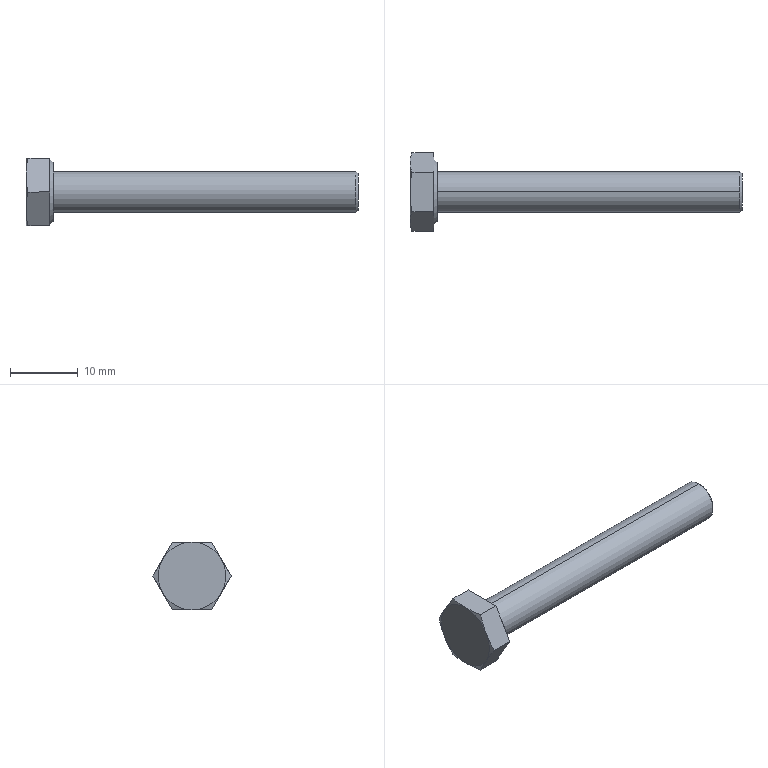Part | SolidWorks | features RevCut 3, Boss 1, Chamfer 1, Extrusion 1, Fillet 1, LPattern 1 | 1 solid | 22 faces | box 49 x 11.547 x 10 mm | volume 1608 mm3 | cone 10 | plane 10 | cylinder 2 | commonest cylinder face diameters 6 x2
STEP:
#1=CARTESIAN_POINT('',(49.,0.,-2.7));
#2=VERTEX_POINT('',#1);
#3=CARTESIAN_POINT('',(49.,0.,2.7));
#4=VERTEX_POINT('',#3);
#5=CARTESIAN_POINT('',(49.,0.,0.));
#6=DIRECTION('',(1.,0.,0.));
#7=DIRECTION('',(0.,0.,-1.));
#8=AXIS2_PLACEMENT_3D('',#5,#6,#7);
#9=CIRCLE('',#8,2.7);
#10=EDGE_CURVE('',#2,#4,#9,.T.);
#11=ORIENTED_EDGE('',*,*,#10,.F.);
#12=CARTESIAN_POINT('',(48.7,0.,-3.));
#13=VERTEX_POINT('',#12);
#14=CARTESIAN_POINT('',(49.,0.,-2.7));
#15=DIRECTION('',(-0.7071,0.,-0.7071));
#16=VECTOR('',#15,1000.);
#17=LINE('',#14,#16);
#18=EDGE_CURVE('',#2,#13,#17,.T.);
#19=ORIENTED_EDGE('',*,*,#18,.T.);
#20=CARTESIAN_POINT('',(48.7,0.,3.));
#21=VERTEX_POINT('',#20);
#22=CARTESIAN_POINT('',(48.7,0.,0.));
#23=DIRECTION('',(-1.,0.,0.));
#24=DIRECTION('',(0.,0.,-1.));
#25=AXIS2_PLACEMENT_3D('',#22,#23,#24);
#26=CIRCLE('',#25,3.);
#27=EDGE_CURVE('',#21,#13,#26,.T.);
#28=ORIENTED_EDGE('',*,*,#27,.F.);
#29=CARTESIAN_POINT('',(49.,0.,2.7));
#30=DIRECTION('',(-0.7071,0.,0.7071));
#31=VECTOR('',#30,1000.);
#32=LINE('',#29,#31);
#33=EDGE_CURVE('',#4,#21,#32,.T.);
#34=ORIENTED_EDGE('',*,*,#33,.F.);
#35=EDGE_LOOP('',(#11,#19,#28,#34));
#36=FACE_OUTER_BOUND('',#35,.T.);
#37=CARTESIAN_POINT('',(49.,0.,0.));
#38=DIRECTION('',(-1.,0.,0.));
#39=DIRECTION('',(0.,0.,1.));
#40=AXIS2_PLACEMENT_3D('',#37,#38,#39);
#41=CONICAL_SURFACE('',#40,2.7,0.7854);
#42=ADVANCED_FACE('',(#36),#41,.T.);
#43=ORIENTED_EDGE('',*,*,#27,.T.);
#44=CARTESIAN_POINT('',(4.,0.,-3.));
#45=VERTEX_POINT('',#44);
#46=CARTESIAN_POINT('',(49.,0.,-3.));
#47=DIRECTION('',(-1.,0.,0.));
#48=VECTOR('',#47,1000.);
#49=LINE('',#46,#48);
#50=EDGE_CURVE('',#13,#45,#49,.T.);
#51=ORIENTED_EDGE('',*,*,#50,.T.);
#52=CARTESIAN_POINT('',(4.,0.,3.));
#53=VERTEX_POINT('',#52);
#54=CARTESIAN_POINT('',(4.,0.,0.));
#55=DIRECTION('',(1.,0.,0.));
#56=DIRECTION('',(0.,0.,1.));
#57=AXIS2_PLACEMENT_3D('',#54,#55,#56);
#58=CIRCLE('',#57,3.);
#59=EDGE_CURVE('',#45,#53,#58,.T.);
#60=ORIENTED_EDGE('',*,*,#59,.T.);
#61=CARTESIAN_POINT('',(49.,0.,3.));
#62=DIRECTION('',(-1.,0.,0.));
#63=VECTOR('',#62,1000.);
#64=LINE('',#61,#63);
#65=EDGE_CURVE('',#21,#53,#64,.T.);
#66=ORIENTED_EDGE('',*,*,#65,.F.);
#67=EDGE_LOOP('',(#43,#51,#60,#66));
#68=FACE_OUTER_BOUND('',#67,.T.);
#69=CARTESIAN_POINT('',(49.,0.,0.));
#70=DIRECTION('',(-1.,0.,0.));
#71=DIRECTION('',(0.,0.,1.));
#72=AXIS2_PLACEMENT_3D('',#69,#70,#71);
#73=CYLINDRICAL_SURFACE('',#72,3.);
#74=ADVANCED_FACE('',(#68),#73,.T.);
#75=CARTESIAN_POINT('',(4.,0.,4.37));
#76=VERTEX_POINT('',#75);
#77=CARTESIAN_POINT('',(4.,0.,-4.37));
#78=VERTEX_POINT('',#77);
#79=CARTESIAN_POINT('',(4.,0.,0.));
#80=DIRECTION('',(-1.,0.,0.));
#81=DIRECTION('',(0.,0.,1.));
#82=AXIS2_PLACEMENT_3D('',#79,#80,#81);
#83=CIRCLE('',#82,4.37);
#84=EDGE_CURVE('',#76,#78,#83,.T.);
#85=ORIENTED_EDGE('',*,*,#84,.T.);
#86=CARTESIAN_POINT('',(3.5,0.,-4.87));
#87=VERTEX_POINT('',#86);
#88=CARTESIAN_POINT('',(3.5,0.,-4.87));
#89=DIRECTION('',(-0.7071,0.,-0.7071));
#90=VECTOR('',#89,1000.);
#91=LINE('',#88,#90);
#92=EDGE_CURVE('',#78,#87,#91,.T.);
#93=ORIENTED_EDGE('',*,*,#92,.T.);
#94=CARTESIAN_POINT('',(3.5,0.,4.87));
#95=VERTEX_POINT('',#94);
#96=CARTESIAN_POINT('',(3.5,0.,0.));
#97=DIRECTION('',(-1.,0.,0.));
#98=DIRECTION('',(0.,0.,1.));
#99=AXIS2_PLACEMENT_3D('',#96,#97,#98);
#100=CIRCLE('',#99,4.87);
#101=EDGE_CURVE('',#95,#87,#100,.T.);
#102=ORIENTED_EDGE('',*,*,#101,.F.);
#103=CARTESIAN_POINT('',(3.5,0.,4.87));
#104=DIRECTION('',(-0.7071,0.,0.7071));
#105=VECTOR('',#104,1000.);
#106=LINE('',#103,#105);
#107=EDGE_CURVE('',#76,#95,#106,.T.);
#108=ORIENTED_EDGE('',*,*,#107,.F.);
#109=EDGE_LOOP('',(#85,#93,#102,#108));
#110=FACE_OUTER_BOUND('',#109,.T.);
#111=CARTESIAN_POINT('',(3.5,0.,0.));
#112=DIRECTION('',(-1.,0.,0.));
#113=DIRECTION('',(0.,0.,1.));
#114=AXIS2_PLACEMENT_3D('',#111,#112,#113);
#115=CONICAL_SURFACE('',#114,4.87,0.7854);
#116=ADVANCED_FACE('',(#110),#115,.T.);
#117=ORIENTED_EDGE('',*,*,#84,.F.);
#118=CARTESIAN_POINT('',(4.,0.,0.));
#119=DIRECTION('',(-1.,0.,0.));
#120=DIRECTION('',(0.,0.,1.));
#121=AXIS2_PLACEMENT_3D('',#118,#119,#120);
#122=CIRCLE('',#121,4.37);
#123=EDGE_CURVE('',#78,#76,#122,.T.);
#124=ORIENTED_EDGE('',*,*,#123,.F.);
#125=EDGE_LOOP('',(#117,#124));
#126=FACE_OUTER_BOUND('',#125,.T.);
#127=CARTESIAN_POINT('',(4.,0.,0.));
#128=DIRECTION('',(1.,0.,0.));
#129=DIRECTION('',(0.,0.,1.));
#130=AXIS2_PLACEMENT_3D('',#127,#128,#129);
#131=CIRCLE('',#130,3.);
#132=EDGE_CURVE('',#53,#45,#131,.T.);
#133=ORIENTED_EDGE('',*,*,#132,.F.);
#134=ORIENTED_EDGE('',*,*,#59,.F.);
#135=EDGE_LOOP('',(#133,#134));
#136=FACE_BOUND('',#135,.T.);
#137=CARTESIAN_POINT('',(4.,-2.887,5.));
#138=DIRECTION('',(-1.,0.,0.));
#139=DIRECTION('',(0.,0.,1.));
#140=AXIS2_PLACEMENT_3D('',#137,#138,#139);
#141=PLANE('',#140);
#142=ADVANCED_FACE('',(#126,#136),#141,.F.);
#143=CARTESIAN_POINT('',(0.2815,-5.774,0.));
#144=VERTEX_POINT('',#143);
#145=CARTESIAN_POINT('',(0.,-4.33,2.5));
#146=VERTEX_POINT('',#145);
#147=CARTESIAN_POINT('',(0.2815,-5.774,0.));
#148=CARTESIAN_POINT('',(0.1064,-5.292,0.8333));
#149=CARTESIAN_POINT('',(0.,-4.811,1.667));
#150=CARTESIAN_POINT('',(0.,-4.33,2.5));
#151=B_SPLINE_CURVE_WITH_KNOTS('',3,(#147,#148,#149,#150),.UNSPECIFIED.,.F.,.F.,(4,4),(0.000000231,0.002887),.UNSPECIFIED.);
#152=EDGE_CURVE('',#144,#146,#151,.T.);
#153=ORIENTED_EDGE('',*,*,#152,.F.);
#154=CARTESIAN_POINT('',(3.5,-5.774,0.));
#155=VERTEX_POINT('',#154);
#156=CARTESIAN_POINT('',(4.,-5.774,0.));
#157=DIRECTION('',(-1.,0.,0.));
#158=VECTOR('',#157,1000.);
#159=LINE('',#156,#158);
#160=EDGE_CURVE('',#155,#144,#159,.T.);
#161=ORIENTED_EDGE('',*,*,#160,.F.);
#162=CARTESIAN_POINT('',(3.5,-2.887,5.));
#163=VERTEX_POINT('',#162);
#164=CARTESIAN_POINT('',(3.5,-2.887,5.));
#165=DIRECTION('',(0.,-0.5,-0.866));
#166=VECTOR('',#165,1000.);
#167=LINE('',#164,#166);
#168=EDGE_CURVE('',#163,#155,#167,.T.);
#169=ORIENTED_EDGE('',*,*,#168,.F.);
#170=CARTESIAN_POINT('',(0.2815,-2.887,5.));
#171=VERTEX_POINT('',#170);
#172=CARTESIAN_POINT('',(4.,-2.887,5.));
#173=DIRECTION('',(-1.,0.,0.));
#174=VECTOR('',#173,1000.);
#175=LINE('',#172,#174);
#176=EDGE_CURVE('',#163,#171,#175,.T.);
#177=ORIENTED_EDGE('',*,*,#176,.T.);
#178=CARTESIAN_POINT('',(0.,-4.33,2.5));
#179=CARTESIAN_POINT('',(0.,-3.849,3.333));
#180=CARTESIAN_POINT('',(0.1064,-3.368,4.167));
#181=CARTESIAN_POINT('',(0.2815,-2.887,5.));
#182=B_SPLINE_CURVE_WITH_KNOTS('',3,(#178,#179,#180,#181),.UNSPECIFIED.,.F.,.F.,(4,4),(0.002887,0.005774),.UNSPECIFIED.);
#183=EDGE_CURVE('',#146,#171,#182,.T.);
#184=ORIENTED_EDGE('',*,*,#183,.F.);
#185=EDGE_LOOP('',(#153,#161,#169,#177,#184));
#186=FACE_OUTER_BOUND('',#185,.T.);
#187=CARTESIAN_POINT('',(4.,-2.887,5.));
#188=DIRECTION('',(0.,0.866,-0.5));
#189=DIRECTION('',(0.,0.5,0.866));
#190=AXIS2_PLACEMENT_3D('',#187,#188,#189);
#191=PLANE('',#190);
#192=ADVANCED_FACE('',(#186),#191,.F.);
#193=CARTESIAN_POINT('',(0.2815,-2.887,-5.));
#194=VERTEX_POINT('',#193);
#195=CARTESIAN_POINT('',(0.,-4.33,-2.5));
#196=VERTEX_POINT('',#195);
#197=CARTESIAN_POINT('',(0.2815,-2.887,-5.));
#198=CARTESIAN_POINT('',(0.1064,-3.368,-4.167));
#199=CARTESIAN_POINT('',(0.,-3.849,-3.333));
#200=CARTESIAN_POINT('',(0.,-4.33,-2.5));
#201=B_SPLINE_CURVE_WITH_KNOTS('',3,(#197,#198,#199,#200),.UNSPECIFIED.,.F.,.F.,(4,4),(0.000000231,0.002887),.UNSPECIFIED.);
#202=EDGE_CURVE('',#194,#196,#201,.T.);
#203=ORIENTED_EDGE('',*,*,#202,.F.);
#204=CARTESIAN_POINT('',(3.5,-2.887,-5.));
#205=VERTEX_POINT('',#204);
#206=CARTESIAN_POINT('',(4.,-2.887,-5.));
#207=DIRECTION('',(-1.,0.,0.));
#208=VECTOR('',#207,1000.);
#209=LINE('',#206,#208);
#210=EDGE_CURVE('',#205,#194,#209,.T.);
#211=ORIENTED_EDGE('',*,*,#210,.F.);
#212=CARTESIAN_POINT('',(3.5,-5.774,0.));
#213=DIRECTION('',(0.,0.5,-0.866));
#214=VECTOR('',#213,1000.);
#215=LINE('',#212,#214);
#216=EDGE_CURVE('',#155,#205,#215,.T.);
#217=ORIENTED_EDGE('',*,*,#216,.F.);
#218=ORIENTED_EDGE('',*,*,#160,.T.);
#219=CARTESIAN_POINT('',(0.,-4.33,-2.5));
#220=CARTESIAN_POINT('',(0.,-4.811,-1.667));
#221=CARTESIAN_POINT('',(0.1064,-5.292,-0.8333));
#222=CARTESIAN_POINT('',(0.2815,-5.774,0.));
#223=B_SPLINE_CURVE_WITH_KNOTS('',3,(#219,#220,#221,#222),.UNSPECIFIED.,.F.,.F.,(4,4),(0.002887,0.005774),.UNSPECIFIED.);
#224=EDGE_CURVE('',#196,#144,#223,.T.);
#225=ORIENTED_EDGE('',*,*,#224,.F.);
#226=EDGE_LOOP('',(#203,#211,#217,#218,#225));
#227=FACE_OUTER_BOUND('',#226,.T.);
#228=CARTESIAN_POINT('',(4.,-5.774,0.));
#229=DIRECTION('',(0.,0.866,0.5));
#230=DIRECTION('',(0.,-0.5,0.866));
#231=AXIS2_PLACEMENT_3D('',#228,#229,#230);
#232=PLANE('',#231);
#233=ADVANCED_FACE('',(#227),#232,.F.);
#234=CARTESIAN_POINT('',(0.2815,2.887,-5.));
#235=VERTEX_POINT('',#234);
#236=CARTESIAN_POINT('',(0.,0.,-5.));
#237=VERTEX_POINT('',#236);
#238=CARTESIAN_POINT('',(0.2815,2.887,-5.));
#239=CARTESIAN_POINT('',(0.1069,1.927,-5.));
#240=CARTESIAN_POINT('',(0.,0.9642,-5.));
#241=CARTESIAN_POINT('',(0.,0.,-5.));
#242=B_SPLINE_CURVE_WITH_KNOTS('',3,(#238,#239,#240,#241),.UNSPECIFIED.,.F.,.F.,(4,4),(0.01041,0.01332),.UNSPECIFIED.);
#243=EDGE_CURVE('',#235,#237,#242,.T.);
#244=ORIENTED_EDGE('',*,*,#243,.F.);
#245=CARTESIAN_POINT('',(3.5,2.887,-5.));
#246=VERTEX_POINT('',#245);
#247=CARTESIAN_POINT('',(4.,2.887,-5.));
#248=DIRECTION('',(-1.,0.,0.));
#249=VECTOR('',#248,1000.);
#250=LINE('',#247,#249);
#251=EDGE_CURVE('',#246,#235,#250,.T.);
#252=ORIENTED_EDGE('',*,*,#251,.F.);
#253=CARTESIAN_POINT('',(3.5,-2.887,-5.));
#254=DIRECTION('',(0.,1.,0.));
#255=VECTOR('',#254,1000.);
#256=LINE('',#253,#255);
#257=EDGE_CURVE('',#205,#246,#256,.T.);
#258=ORIENTED_EDGE('',*,*,#257,.F.);
#259=ORIENTED_EDGE('',*,*,#210,.T.);
#260=CARTESIAN_POINT('',(0.,0.,-5.));
#261=CARTESIAN_POINT('',(0.,-0.4807,-5.));
#262=CARTESIAN_POINT('',(0.02571,-0.962,-5.));
#263=CARTESIAN_POINT('',(0.123,-1.926,-5.));
#264=CARTESIAN_POINT('',(0.1945,-2.409,-5.));
#265=CARTESIAN_POINT('',(0.2815,-2.887,-5.));
#266=B_SPLINE_CURVE_WITH_KNOTS('',3,(#260,#261,#262,#263,#264,#265),.UNSPECIFIED.,.F.,.F.,(4,2,4),(0.01332,0.01477,0.01622),.UNSPECIFIED.);
#267=EDGE_CURVE('',#237,#194,#266,.T.);
#268=ORIENTED_EDGE('',*,*,#267,.F.);
#269=EDGE_LOOP('',(#244,#252,#258,#259,#268));
#270=FACE_OUTER_BOUND('',#269,.T.);
#271=CARTESIAN_POINT('',(4.,-2.887,-5.));
#272=DIRECTION('',(0.,0.,1.));
#273=DIRECTION('',(0.,-1.,0.));
#274=AXIS2_PLACEMENT_3D('',#271,#272,#273);
#275=PLANE('',#274);
#276=ADVANCED_FACE('',(#270),#275,.F.);
#277=CARTESIAN_POINT('',(0.2815,5.774,0.));
#278=VERTEX_POINT('',#277);
#279=CARTESIAN_POINT('',(0.,4.33,-2.5));
#280=VERTEX_POINT('',#279);
#281=CARTESIAN_POINT('',(0.2815,5.774,0.));
#282=CARTESIAN_POINT('',(0.1064,5.292,-0.8333));
#283=CARTESIAN_POINT('',(0.,4.811,-1.667));
#284=CARTESIAN_POINT('',(0.,4.33,-2.5));
#285=B_SPLINE_CURVE_WITH_KNOTS('',3,(#281,#282,#283,#284),.UNSPECIFIED.,.F.,.F.,(4,4),(0.000000231,0.002887),.UNSPECIFIED.);
#286=EDGE_CURVE('',#278,#280,#285,.T.);
#287=ORIENTED_EDGE('',*,*,#286,.F.);
#288=CARTESIAN_POINT('',(3.5,5.774,0.));
#289=VERTEX_POINT('',#288);
#290=CARTESIAN_POINT('',(4.,5.774,0.));
#291=DIRECTION('',(-1.,0.,0.));
#292=VECTOR('',#291,1000.);
#293=LINE('',#290,#292);
#294=EDGE_CURVE('',#289,#278,#293,.T.);
#295=ORIENTED_EDGE('',*,*,#294,.F.);
#296=CARTESIAN_POINT('',(3.5,2.887,-5.));
#297=DIRECTION('',(0.,0.5,0.866));
#298=VECTOR('',#297,1000.);
#299=LINE('',#296,#298);
#300=EDGE_CURVE('',#246,#289,#299,.T.);
#301=ORIENTED_EDGE('',*,*,#300,.F.);
#302=ORIENTED_EDGE('',*,*,#251,.T.);
#303=CARTESIAN_POINT('',(0.,4.33,-2.5));
#304=CARTESIAN_POINT('',(0.,3.849,-3.333));
#305=CARTESIAN_POINT('',(0.1064,3.368,-4.167));
#306=CARTESIAN_POINT('',(0.2815,2.887,-5.));
#307=B_SPLINE_CURVE_WITH_KNOTS('',3,(#303,#304,#305,#306),.UNSPECIFIED.,.F.,.F.,(4,4),(0.002887,0.005774),.UNSPECIFIED.);
#308=EDGE_CURVE('',#280,#235,#307,.T.);
#309=ORIENTED_EDGE('',*,*,#308,.F.);
#310=EDGE_LOOP('',(#287,#295,#301,#302,#309));
#311=FACE_OUTER_BOUND('',#310,.T.);
#312=CARTESIAN_POINT('',(4.,2.887,-5.));
#313=DIRECTION('',(0.,-0.866,0.5));
#314=DIRECTION('',(0.,-0.5,-0.866));
#315=AXIS2_PLACEMENT_3D('',#312,#313,#314);
#316=PLANE('',#315);
#317=ADVANCED_FACE('',(#311),#316,.F.);
#318=CARTESIAN_POINT('',(0.2815,2.887,5.));
#319=VERTEX_POINT('',#318);
#320=CARTESIAN_POINT('',(0.,4.33,2.5));
#321=VERTEX_POINT('',#320);
#322=CARTESIAN_POINT('',(0.2815,2.887,5.));
#323=CARTESIAN_POINT('',(0.1064,3.368,4.167));
#324=CARTESIAN_POINT('',(0.,3.849,3.333));
#325=CARTESIAN_POINT('',(0.,4.33,2.5));
#326=B_SPLINE_CURVE_WITH_KNOTS('',3,(#322,#323,#324,#325),.UNSPECIFIED.,.F.,.F.,(4,4),(0.000000231,0.002887),.UNSPECIFIED.);
#327=EDGE_CURVE('',#319,#321,#326,.T.);
#328=ORIENTED_EDGE('',*,*,#327,.F.);
#329=CARTESIAN_POINT('',(3.5,2.887,5.));
#330=VERTEX_POINT('',#329);
#331=CARTESIAN_POINT('',(4.,2.887,5.));
#332=DIRECTION('',(-1.,0.,0.));
#333=VECTOR('',#332,1000.);
#334=LINE('',#331,#333);
#335=EDGE_CURVE('',#330,#319,#334,.T.);
#336=ORIENTED_EDGE('',*,*,#335,.F.);
#337=CARTESIAN_POINT('',(3.5,5.774,0.));
#338=DIRECTION('',(0.,-0.5,0.866));
#339=VECTOR('',#338,1000.);
#340=LINE('',#337,#339);
#341=EDGE_CURVE('',#289,#330,#340,.T.);
#342=ORIENTED_EDGE('',*,*,#341,.F.);
#343=ORIENTED_EDGE('',*,*,#294,.T.);
#344=CARTESIAN_POINT('',(0.,4.33,2.5));
#345=CARTESIAN_POINT('',(0.,4.811,1.667));
#346=CARTESIAN_POINT('',(0.1064,5.292,0.8333));
#347=CARTESIAN_POINT('',(0.2815,5.774,0.));
#348=B_SPLINE_CURVE_WITH_KNOTS('',3,(#344,#345,#346,#347),.UNSPECIFIED.,.F.,.F.,(4,4),(0.002887,0.005774),.UNSPECIFIED.);
#349=EDGE_CURVE('',#321,#278,#348,.T.);
#350=ORIENTED_EDGE('',*,*,#349,.F.);
#351=EDGE_LOOP('',(#328,#336,#342,#343,#350));
#352=FACE_OUTER_BOUND('',#351,.T.);
#353=CARTESIAN_POINT('',(4.,5.774,0.));
#354=DIRECTION('',(0.,-0.866,-0.5));
#355=DIRECTION('',(0.,0.5,-0.866));
#356=AXIS2_PLACEMENT_3D('',#353,#354,#355);
#357=PLANE('',#356);
#358=ADVANCED_FACE('',(#352),#357,.F.);
#359=CARTESIAN_POINT('',(0.,0.,5.));
#360=VERTEX_POINT('',#359);
#361=CARTESIAN_POINT('',(0.2815,-2.887,5.));
#362=CARTESIAN_POINT('',(0.1945,-2.409,5.));
#363=CARTESIAN_POINT('',(0.123,-1.926,5.));
#364=CARTESIAN_POINT('',(0.02571,-0.962,5.));
#365=CARTESIAN_POINT('',(0.,-0.4807,5.));
#366=CARTESIAN_POINT('',(0.,0.,5.));
#367=B_SPLINE_CURVE_WITH_KNOTS('',3,(#361,#362,#363,#364,#365,#366),.UNSPECIFIED.,.F.,.F.,(4,2,4),(0.004911,0.006366,0.00782),.UNSPECIFIED.);
#368=EDGE_CURVE('',#171,#360,#367,.T.);
#369=ORIENTED_EDGE('',*,*,#368,.F.);
#370=ORIENTED_EDGE('',*,*,#176,.F.);
#371=CARTESIAN_POINT('',(3.5,2.887,5.));
#372=DIRECTION('',(0.,-1.,0.));
#373=VECTOR('',#372,1000.);
#374=LINE('',#371,#373);
#375=EDGE_CURVE('',#330,#163,#374,.T.);
#376=ORIENTED_EDGE('',*,*,#375,.F.);
#377=ORIENTED_EDGE('',*,*,#335,.T.);
#378=CARTESIAN_POINT('',(0.,0.,5.));
#379=CARTESIAN_POINT('',(0.,0.9642,5.));
#380=CARTESIAN_POINT('',(0.1069,1.927,5.));
#381=CARTESIAN_POINT('',(0.2815,2.887,5.));
#382=B_SPLINE_CURVE_WITH_KNOTS('',3,(#378,#379,#380,#381),.UNSPECIFIED.,.F.,.F.,(4,4),(0.00782,0.01074),.UNSPECIFIED.);
#383=EDGE_CURVE('',#360,#319,#382,.T.);
#384=ORIENTED_EDGE('',*,*,#383,.F.);
#385=EDGE_LOOP('',(#369,#370,#376,#377,#384));
#386=FACE_OUTER_BOUND('',#385,.T.);
#387=CARTESIAN_POINT('',(4.,2.887,5.));
#388=DIRECTION('',(0.,0.,-1.));
#389=DIRECTION('',(0.,1.,0.));
#390=AXIS2_PLACEMENT_3D('',#387,#388,#389);
#391=PLANE('',#390);
#392=ADVANCED_FACE('',(#386),#391,.F.);
#393=ORIENTED_EDGE('',*,*,#101,.T.);
#394=CARTESIAN_POINT('',(3.5,0.,0.));
#395=DIRECTION('',(-1.,0.,0.));
#396=DIRECTION('',(0.,0.,1.));
#397=AXIS2_PLACEMENT_3D('',#394,#395,#396);
#398=CIRCLE('',#397,4.87);
#399=EDGE_CURVE('',#87,#95,#398,.T.);
#400=ORIENTED_EDGE('',*,*,#399,.T.);
#401=EDGE_LOOP('',(#393,#400));
#402=FACE_BOUND('',#401,.T.);
#403=ORIENTED_EDGE('',*,*,#168,.T.);
#404=ORIENTED_EDGE('',*,*,#216,.T.);
#405=ORIENTED_EDGE('',*,*,#257,.T.);
#406=ORIENTED_EDGE('',*,*,#300,.T.);
#407=ORIENTED_EDGE('',*,*,#341,.T.);
#408=ORIENTED_EDGE('',*,*,#375,.T.);
#409=EDGE_LOOP('',(#403,#404,#405,#406,#407,#408));
#410=FACE_OUTER_BOUND('',#409,.T.);
#411=CARTESIAN_POINT('',(3.5,4.87,0.));
#412=DIRECTION('',(1.,0.,0.));
#413=DIRECTION('',(0.,0.,-1.));
#414=AXIS2_PLACEMENT_3D('',#411,#412,#413);
#415=PLANE('',#414);
#416=ADVANCED_FACE('',(#402,#410),#415,.T.);
#417=ORIENTED_EDGE('',*,*,#92,.F.);
#418=ORIENTED_EDGE('',*,*,#123,.T.);
#419=ORIENTED_EDGE('',*,*,#107,.T.);
#420=ORIENTED_EDGE('',*,*,#399,.F.);
#421=EDGE_LOOP('',(#417,#418,#419,#420));
#422=FACE_OUTER_BOUND('',#421,.T.);
#423=CARTESIAN_POINT('',(3.5,0.,0.));
#424=DIRECTION('',(-1.,0.,0.));
#425=DIRECTION('',(0.,0.,1.));
#426=AXIS2_PLACEMENT_3D('',#423,#424,#425);
#427=CONICAL_SURFACE('',#426,4.87,0.7854);
#428=ADVANCED_FACE('',(#422),#427,.T.);
#429=ORIENTED_EDGE('',*,*,#183,.T.);
#430=ORIENTED_EDGE('',*,*,#368,.T.);
#431=CARTESIAN_POINT('',(0.,0.,0.));
#432=DIRECTION('',(-1.,0.,0.));
#433=DIRECTION('',(0.,0.,1.));
#434=AXIS2_PLACEMENT_3D('',#431,#432,#433);
#435=CIRCLE('',#434,5.);
#436=EDGE_CURVE('',#146,#360,#435,.T.);
#437=ORIENTED_EDGE('',*,*,#436,.F.);
#438=EDGE_LOOP('',(#429,#430,#437));
#439=FACE_OUTER_BOUND('',#438,.T.);
#440=CARTESIAN_POINT('',(0.,0.,0.));
#441=DIRECTION('',(1.,0.,0.));
#442=DIRECTION('',(0.,0.,-1.));
#443=AXIS2_PLACEMENT_3D('',#440,#441,#442);
#444=CONICAL_SURFACE('',#443,5.,1.222);
#445=ADVANCED_FACE('',(#439),#444,.T.);
#446=ORIENTED_EDGE('',*,*,#224,.T.);
#447=ORIENTED_EDGE('',*,*,#152,.T.);
#448=CARTESIAN_POINT('',(0.,0.,0.));
#449=DIRECTION('',(-1.,0.,0.));
#450=DIRECTION('',(0.,0.,1.));
#451=AXIS2_PLACEMENT_3D('',#448,#449,#450);
#452=CIRCLE('',#451,5.);
#453=EDGE_CURVE('',#196,#146,#452,.T.);
#454=ORIENTED_EDGE('',*,*,#453,.F.);
#455=EDGE_LOOP('',(#446,#447,#454));
#456=FACE_OUTER_BOUND('',#455,.T.);
#457=CARTESIAN_POINT('',(0.,0.,0.));
#458=DIRECTION('',(1.,0.,0.));
#459=DIRECTION('',(0.,0.,-1.));
#460=AXIS2_PLACEMENT_3D('',#457,#458,#459);
#461=CONICAL_SURFACE('',#460,5.,1.222);
#462=ADVANCED_FACE('',(#456),#461,.T.);
#463=ORIENTED_EDGE('',*,*,#267,.T.);
#464=ORIENTED_EDGE('',*,*,#202,.T.);
#465=CARTESIAN_POINT('',(0.,0.,0.));
#466=DIRECTION('',(-1.,0.,0.));
#467=DIRECTION('',(0.,0.,1.));
#468=AXIS2_PLACEMENT_3D('',#465,#466,#467);
#469=CIRCLE('',#468,5.);
#470=EDGE_CURVE('',#237,#196,#469,.T.);
#471=ORIENTED_EDGE('',*,*,#470,.F.);
#472=EDGE_LOOP('',(#463,#464,#471));
#473=FACE_OUTER_BOUND('',#472,.T.);
#474=CARTESIAN_POINT('',(0.,0.,0.));
#475=DIRECTION('',(1.,0.,0.));
#476=DIRECTION('',(0.,0.,-1.));
#477=AXIS2_PLACEMENT_3D('',#474,#475,#476);
#478=CONICAL_SURFACE('',#477,5.,1.222);
#479=ADVANCED_FACE('',(#473),#478,.T.);
#480=ORIENTED_EDGE('',*,*,#243,.T.);
#481=CARTESIAN_POINT('',(0.,0.,0.));
#482=DIRECTION('',(-1.,0.,0.));
#483=DIRECTION('',(0.,0.,1.));
#484=AXIS2_PLACEMENT_3D('',#481,#482,#483);
#485=CIRCLE('',#484,5.);
#486=EDGE_CURVE('',#280,#237,#485,.T.);
#487=ORIENTED_EDGE('',*,*,#486,.F.);
#488=ORIENTED_EDGE('',*,*,#308,.T.);
#489=EDGE_LOOP('',(#480,#487,#488));
#490=FACE_OUTER_BOUND('',#489,.T.);
#491=CARTESIAN_POINT('',(0.,0.,0.));
#492=DIRECTION('',(1.,0.,0.));
#493=DIRECTION('',(0.,0.,-1.));
#494=AXIS2_PLACEMENT_3D('',#491,#492,#493);
#495=CONICAL_SURFACE('',#494,5.,1.222);
#496=ADVANCED_FACE('',(#490),#495,.T.);
#497=ORIENTED_EDGE('',*,*,#286,.T.);
#498=CARTESIAN_POINT('',(0.,0.,0.));
#499=DIRECTION('',(-1.,0.,0.));
#500=DIRECTION('',(0.,0.,1.));
#501=AXIS2_PLACEMENT_3D('',#498,#499,#500);
#502=CIRCLE('',#501,5.);
#503=EDGE_CURVE('',#321,#280,#502,.T.);
#504=ORIENTED_EDGE('',*,*,#503,.F.);
#505=ORIENTED_EDGE('',*,*,#349,.T.);
#506=EDGE_LOOP('',(#497,#504,#505));
#507=FACE_OUTER_BOUND('',#506,.T.);
#508=CARTESIAN_POINT('',(0.,0.,0.));
#509=DIRECTION('',(1.,0.,0.));
#510=DIRECTION('',(0.,0.,-1.));
#511=AXIS2_PLACEMENT_3D('',#508,#509,#510);
#512=CONICAL_SURFACE('',#511,5.,1.222);
#513=ADVANCED_FACE('',(#507),#512,.T.);
#514=ORIENTED_EDGE('',*,*,#327,.T.);
#515=CARTESIAN_POINT('',(0.,0.,0.));
#516=DIRECTION('',(-1.,0.,0.));
#517=DIRECTION('',(0.,0.,1.));
#518=AXIS2_PLACEMENT_3D('',#515,#516,#517);
#519=CIRCLE('',#518,5.);
#520=EDGE_CURVE('',#360,#321,#519,.T.);
#521=ORIENTED_EDGE('',*,*,#520,.F.);
#522=ORIENTED_EDGE('',*,*,#383,.T.);
#523=EDGE_LOOP('',(#514,#521,#522));
#524=FACE_OUTER_BOUND('',#523,.T.);
#525=CARTESIAN_POINT('',(0.,0.,0.));
#526=DIRECTION('',(1.,0.,0.));
#527=DIRECTION('',(0.,0.,-1.));
#528=AXIS2_PLACEMENT_3D('',#525,#526,#527);
#529=CONICAL_SURFACE('',#528,5.,1.222);
#530=ADVANCED_FACE('',(#524),#529,.T.);
#531=ORIENTED_EDGE('',*,*,#436,.T.);
#532=ORIENTED_EDGE('',*,*,#520,.T.);
#533=ORIENTED_EDGE('',*,*,#503,.T.);
#534=ORIENTED_EDGE('',*,*,#486,.T.);
#535=ORIENTED_EDGE('',*,*,#470,.T.);
#536=ORIENTED_EDGE('',*,*,#453,.T.);
#537=EDGE_LOOP('',(#531,#532,#533,#534,#535,#536));
#538=FACE_OUTER_BOUND('',#537,.T.);
#539=CARTESIAN_POINT('',(0.,-2.887,5.));
#540=DIRECTION('',(-1.,0.,0.));
#541=DIRECTION('',(0.,0.,1.));
#542=AXIS2_PLACEMENT_3D('',#539,#540,#541);
#543=PLANE('',#542);
#544=ADVANCED_FACE('',(#538),#543,.T.);
#545=ORIENTED_EDGE('',*,*,#50,.F.);
#546=CARTESIAN_POINT('',(48.7,0.,0.));
#547=DIRECTION('',(-1.,0.,0.));
#548=DIRECTION('',(0.,0.,-1.));
#549=AXIS2_PLACEMENT_3D('',#546,#547,#548);
#550=CIRCLE('',#549,3.);
#551=EDGE_CURVE('',#13,#21,#550,.T.);
#552=ORIENTED_EDGE('',*,*,#551,.T.);
#553=ORIENTED_EDGE('',*,*,#65,.T.);
#554=ORIENTED_EDGE('',*,*,#132,.T.);
#555=EDGE_LOOP('',(#545,#552,#553,#554));
#556=FACE_OUTER_BOUND('',#555,.T.);
#557=CARTESIAN_POINT('',(49.,0.,0.));
#558=DIRECTION('',(-1.,0.,0.));
#559=DIRECTION('',(0.,0.,1.));
#560=AXIS2_PLACEMENT_3D('',#557,#558,#559);
#561=CYLINDRICAL_SURFACE('',#560,3.);
#562=ADVANCED_FACE('',(#556),#561,.T.);
#563=CARTESIAN_POINT('',(49.,0.,0.));
#564=DIRECTION('',(1.,0.,0.));
#565=DIRECTION('',(0.,0.,-1.));
#566=AXIS2_PLACEMENT_3D('',#563,#564,#565);
#567=CIRCLE('',#566,2.7);
#568=EDGE_CURVE('',#4,#2,#567,.T.);
#569=ORIENTED_EDGE('',*,*,#568,.T.);
#570=ORIENTED_EDGE('',*,*,#10,.T.);
#571=EDGE_LOOP('',(#569,#570));
#572=FACE_OUTER_BOUND('',#571,.T.);
#573=CARTESIAN_POINT('',(49.,0.,0.));
#574=DIRECTION('',(1.,0.,0.));
#575=DIRECTION('',(0.,0.,-1.));
#576=AXIS2_PLACEMENT_3D('',#573,#574,#575);
#577=PLANE('',#576);
#578=ADVANCED_FACE('',(#572),#577,.T.);
#579=ORIENTED_EDGE('',*,*,#18,.F.);
#580=ORIENTED_EDGE('',*,*,#568,.F.);
#581=ORIENTED_EDGE('',*,*,#33,.T.);
#582=ORIENTED_EDGE('',*,*,#551,.F.);
#583=EDGE_LOOP('',(#579,#580,#581,#582));
#584=FACE_OUTER_BOUND('',#583,.T.);
#585=CARTESIAN_POINT('',(49.,0.,0.));
#586=DIRECTION('',(-1.,0.,0.));
#587=DIRECTION('',(0.,0.,1.));
#588=AXIS2_PLACEMENT_3D('',#585,#586,#587);
#589=CONICAL_SURFACE('',#588,2.7,0.7854);
#590=ADVANCED_FACE('',(#584),#589,.T.);
#591=CLOSED_SHELL('',(#42,#74,#116,#142,#192,#233,#276,#317,#358,#392,#416,#428,#445,#462,#479,#496,#513,#530,#544,#562,#578,#590));
#592=MANIFOLD_SOLID_BREP('',#591);
#593=CARTESIAN_POINT('',(0.,0.,0.));
#594=DIRECTION('',(0.,0.,1.));
#595=DIRECTION('',(1.,0.,0.));
#596=AXIS2_PLACEMENT_3D('',#593,#594,#595);
#597=(LENGTH_UNIT()NAMED_UNIT(*)SI_UNIT(.MILLI.,.METRE.));
#598=UNCERTAINTY_MEASURE_WITH_UNIT(LENGTH_MEASURE(0.00001),#597,'','');
#599=(NAMED_UNIT(*)PLANE_ANGLE_UNIT()SI_UNIT($,.RADIAN.));
#600=(NAMED_UNIT(*)SI_UNIT($,.STERADIAN.)SOLID_ANGLE_UNIT());
#601=(GEOMETRIC_REPRESENTATION_CONTEXT(3)GLOBAL_UNCERTAINTY_ASSIGNED_CONTEXT((#598))GLOBAL_UNIT_ASSIGNED_CONTEXT((#597,#599,#600))REPRESENTATION_CONTEXT('',''));
#602=ADVANCED_BREP_SHAPE_REPRESENTATION('',(#592,#596),#601);